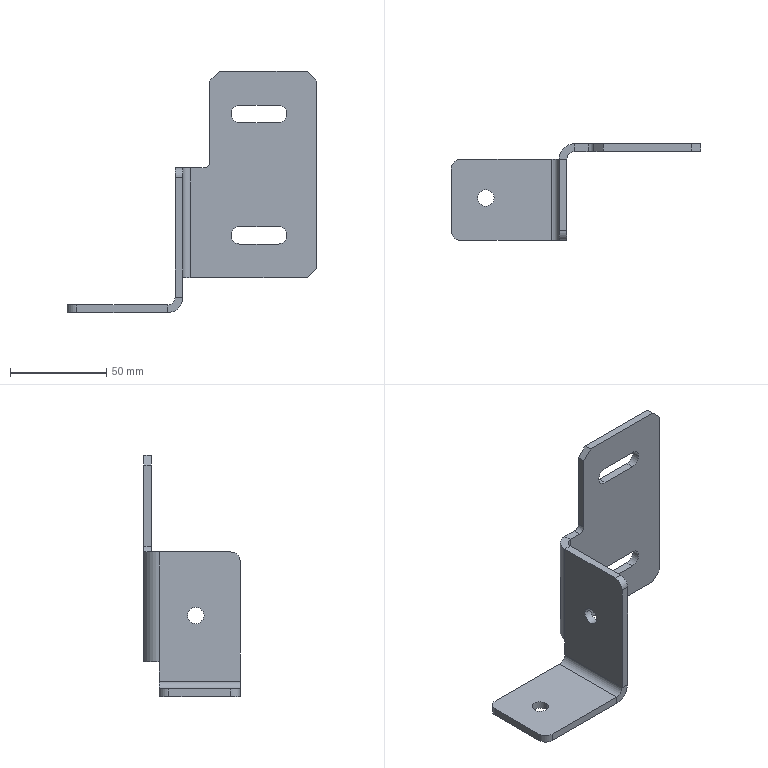Part | SolidWorks | features ICE 4, Fillet 2, Chamfer 1, EdgeFlange 1, FlatPattern 1, SMBaseFlange 1, SheetMetal 1 | 1 solid | 44 faces | box 129.5 x 50 x 125 mm | volume 47149 mm3 | plane 28 | cylinder 16 | commonest cylinder face diameters 8.5 x4 9 x4 10 x3 8 x2 16 x2 6 x1
STEP:
#1=CARTESIAN_POINT('',(-96.75,-28.,-18.));
#2=VERTEX_POINT('',#1);
#3=CARTESIAN_POINT('',(-105.25,-28.,-18.));
#4=VERTEX_POINT('',#3);
#5=CARTESIAN_POINT('',(-101.,-28.,-18.));
#6=DIRECTION('',(0.,0.,-1.));
#7=DIRECTION('',(1.,0.,0.));
#8=AXIS2_PLACEMENT_3D('',#5,#6,#7);
#9=CIRCLE('',#8,4.25);
#10=EDGE_CURVE('',#2,#4,#9,.T.);
#11=ORIENTED_EDGE('',*,*,#10,.T.);
#12=CARTESIAN_POINT('',(-105.25,-28.,-14.));
#13=VERTEX_POINT('',#12);
#14=CARTESIAN_POINT('',(-105.25,-28.,-18.001));
#15=DIRECTION('',(0.,0.,1.));
#16=VECTOR('',#15,1000.);
#17=LINE('',#14,#16);
#18=EDGE_CURVE('',#4,#13,#17,.T.);
#19=ORIENTED_EDGE('',*,*,#18,.T.);
#20=CARTESIAN_POINT('',(-96.75,-28.,-14.));
#21=VERTEX_POINT('',#20);
#22=CARTESIAN_POINT('',(-101.,-28.,-14.));
#23=DIRECTION('',(0.,0.,1.));
#24=DIRECTION('',(1.,0.,0.));
#25=AXIS2_PLACEMENT_3D('',#22,#23,#24);
#26=CIRCLE('',#25,4.25);
#27=EDGE_CURVE('',#13,#21,#26,.T.);
#28=ORIENTED_EDGE('',*,*,#27,.T.);
#29=CARTESIAN_POINT('',(-96.75,-28.,-18.001));
#30=DIRECTION('',(0.,0.,1.));
#31=VECTOR('',#30,1000.);
#32=LINE('',#29,#31);
#33=EDGE_CURVE('',#2,#21,#32,.T.);
#34=ORIENTED_EDGE('',*,*,#33,.F.);
#35=EDGE_LOOP('',(#11,#19,#28,#34));
#36=FACE_OUTER_BOUND('',#35,.T.);
#37=CARTESIAN_POINT('',(-101.,-28.,-18.001));
#38=DIRECTION('',(0.,0.,1.));
#39=DIRECTION('',(1.,0.,0.));
#40=AXIS2_PLACEMENT_3D('',#37,#38,#39);
#41=CYLINDRICAL_SURFACE('',#40,4.25);
#42=ADVANCED_FACE('',(#36),#41,.F.);
#43=CARTESIAN_POINT('',(-59.,-22.75,24.));
#44=VERTEX_POINT('',#43);
#45=CARTESIAN_POINT('',(-59.,-31.25,24.));
#46=VERTEX_POINT('',#45);
#47=CARTESIAN_POINT('',(-59.,-27.,24.));
#48=DIRECTION('',(-1.,0.,0.));
#49=DIRECTION('',(0.,0.,-1.));
#50=AXIS2_PLACEMENT_3D('',#47,#48,#49);
#51=CIRCLE('',#50,4.25);
#52=EDGE_CURVE('',#44,#46,#51,.T.);
#53=ORIENTED_EDGE('',*,*,#52,.F.);
#54=CARTESIAN_POINT('',(-63.,-22.75,24.));
#55=VERTEX_POINT('',#54);
#56=CARTESIAN_POINT('',(10.501,-22.75,24.));
#57=DIRECTION('',(-1.,0.,0.));
#58=VECTOR('',#57,1000.);
#59=LINE('',#56,#58);
#60=EDGE_CURVE('',#44,#55,#59,.T.);
#61=ORIENTED_EDGE('',*,*,#60,.T.);
#62=CARTESIAN_POINT('',(-63.,-31.25,24.));
#63=VERTEX_POINT('',#62);
#64=CARTESIAN_POINT('',(-63.,-27.,24.));
#65=DIRECTION('',(-1.,0.,0.));
#66=DIRECTION('',(0.,-1.,0.));
#67=AXIS2_PLACEMENT_3D('',#64,#65,#66);
#68=CIRCLE('',#67,4.25);
#69=EDGE_CURVE('',#55,#63,#68,.T.);
#70=ORIENTED_EDGE('',*,*,#69,.T.);
#71=CARTESIAN_POINT('',(10.501,-31.25,24.));
#72=DIRECTION('',(-1.,0.,0.));
#73=VECTOR('',#72,1000.);
#74=LINE('',#71,#73);
#75=EDGE_CURVE('',#46,#63,#74,.T.);
#76=ORIENTED_EDGE('',*,*,#75,.F.);
#77=EDGE_LOOP('',(#53,#61,#70,#76));
#78=FACE_OUTER_BOUND('',#77,.T.);
#79=CARTESIAN_POINT('',(10.501,-27.,24.));
#80=DIRECTION('',(-1.,0.,0.));
#81=DIRECTION('',(0.,-1.,0.));
#82=AXIS2_PLACEMENT_3D('',#79,#80,#81);
#83=CYLINDRICAL_SURFACE('',#82,4.25);
#84=ADVANCED_FACE('',(#78),#83,.F.);
#85=CARTESIAN_POINT('',(-48.,-4.,57.));
#86=VERTEX_POINT('',#85);
#87=CARTESIAN_POINT('',(-55.,-4.,57.));
#88=VERTEX_POINT('',#87);
#89=CARTESIAN_POINT('',(-63.,-4.,57.));
#90=DIRECTION('',(-1.,0.,0.));
#91=VECTOR('',#90,1000.);
#92=LINE('',#89,#91);
#93=EDGE_CURVE('',#86,#88,#92,.T.);
#94=ORIENTED_EDGE('',*,*,#93,.F.);
#95=CARTESIAN_POINT('',(-48.,0.,57.));
#96=VERTEX_POINT('',#95);
#97=CARTESIAN_POINT('',(-48.,0.,57.));
#98=DIRECTION('',(0.,1.,0.));
#99=VECTOR('',#98,1000.);
#100=LINE('',#97,#99);
#101=EDGE_CURVE('',#86,#96,#100,.T.);
#102=ORIENTED_EDGE('',*,*,#101,.T.);
#103=CARTESIAN_POINT('',(-55.,0.,57.));
#104=VERTEX_POINT('',#103);
#105=CARTESIAN_POINT('',(-63.,0.,57.));
#106=DIRECTION('',(1.,0.,0.));
#107=VECTOR('',#106,1000.);
#108=LINE('',#105,#107);
#109=EDGE_CURVE('',#104,#96,#108,.T.);
#110=ORIENTED_EDGE('',*,*,#109,.F.);
#111=CARTESIAN_POINT('',(-55.,0.,57.));
#112=DIRECTION('',(0.,-1.,0.));
#113=VECTOR('',#112,1000.);
#114=LINE('',#111,#113);
#115=EDGE_CURVE('',#104,#88,#114,.T.);
#116=ORIENTED_EDGE('',*,*,#115,.T.);
#117=EDGE_LOOP('',(#94,#102,#110,#116));
#118=FACE_OUTER_BOUND('',#117,.T.);
#119=CARTESIAN_POINT('',(-63.,-50.,57.));
#120=DIRECTION('',(0.,0.,1.));
#121=DIRECTION('',(1.,0.,0.));
#122=AXIS2_PLACEMENT_3D('',#119,#120,#121);
#123=PLANE('',#122);
#124=ADVANCED_FACE('',(#118),#123,.T.);
#125=CARTESIAN_POINT('',(-63.,-45.,57.));
#126=VERTEX_POINT('',#125);
#127=CARTESIAN_POINT('',(-63.,-8.,57.));
#128=VERTEX_POINT('',#127);
#129=CARTESIAN_POINT('',(-63.,-50.,57.));
#130=DIRECTION('',(0.,1.,0.));
#131=VECTOR('',#130,1000.);
#132=LINE('',#129,#131);
#133=EDGE_CURVE('',#126,#128,#132,.T.);
#134=ORIENTED_EDGE('',*,*,#133,.F.);
#135=CARTESIAN_POINT('',(-59.,-45.,57.));
#136=VERTEX_POINT('',#135);
#137=CARTESIAN_POINT('',(-63.,-45.,57.));
#138=DIRECTION('',(1.,0.,0.));
#139=VECTOR('',#138,1000.);
#140=LINE('',#137,#139);
#141=EDGE_CURVE('',#126,#136,#140,.T.);
#142=ORIENTED_EDGE('',*,*,#141,.T.);
#143=CARTESIAN_POINT('',(-59.,-8.,57.));
#144=VERTEX_POINT('',#143);
#145=CARTESIAN_POINT('',(-59.,0.,57.));
#146=DIRECTION('',(0.,-1.,0.));
#147=VECTOR('',#146,1000.);
#148=LINE('',#145,#147);
#149=EDGE_CURVE('',#144,#136,#148,.T.);
#150=ORIENTED_EDGE('',*,*,#149,.F.);
#151=CARTESIAN_POINT('',(-59.,-8.,57.));
#152=DIRECTION('',(-1.,0.,0.));
#153=VECTOR('',#152,1000.);
#154=LINE('',#151,#153);
#155=EDGE_CURVE('',#144,#128,#154,.T.);
#156=ORIENTED_EDGE('',*,*,#155,.T.);
#157=EDGE_LOOP('',(#134,#142,#150,#156));
#158=FACE_OUTER_BOUND('',#157,.T.);
#159=CARTESIAN_POINT('',(-63.,-50.,57.));
#160=DIRECTION('',(0.,0.,1.));
#161=DIRECTION('',(1.,0.,0.));
#162=AXIS2_PLACEMENT_3D('',#159,#160,#161);
#163=PLANE('',#162);
#164=ADVANCED_FACE('',(#158),#163,.T.);
#165=CARTESIAN_POINT('',(5.5,-4.,107.));
#166=VERTEX_POINT('',#165);
#167=CARTESIAN_POINT('',(-40.,-4.,107.));
#168=VERTEX_POINT('',#167);
#169=CARTESIAN_POINT('',(-63.,-4.,107.));
#170=DIRECTION('',(-1.,0.,0.));
#171=VECTOR('',#170,1000.);
#172=LINE('',#169,#171);
#173=EDGE_CURVE('',#166,#168,#172,.T.);
#174=ORIENTED_EDGE('',*,*,#173,.F.);
#175=CARTESIAN_POINT('',(5.5,0.,107.));
#176=VERTEX_POINT('',#175);
#177=CARTESIAN_POINT('',(5.5,-8.,107.));
#178=DIRECTION('',(0.,1.,0.));
#179=VECTOR('',#178,1000.);
#180=LINE('',#177,#179);
#181=EDGE_CURVE('',#166,#176,#180,.T.);
#182=ORIENTED_EDGE('',*,*,#181,.T.);
#183=CARTESIAN_POINT('',(-40.,0.,107.));
#184=VERTEX_POINT('',#183);
#185=CARTESIAN_POINT('',(-63.,0.,107.));
#186=DIRECTION('',(-1.,0.,0.));
#187=VECTOR('',#186,1000.);
#188=LINE('',#185,#187);
#189=EDGE_CURVE('',#176,#184,#188,.T.);
#190=ORIENTED_EDGE('',*,*,#189,.T.);
#191=CARTESIAN_POINT('',(-40.,-8.,107.));
#192=DIRECTION('',(0.,-1.,0.));
#193=VECTOR('',#192,1000.);
#194=LINE('',#191,#193);
#195=EDGE_CURVE('',#184,#168,#194,.T.);
#196=ORIENTED_EDGE('',*,*,#195,.T.);
#197=EDGE_LOOP('',(#174,#182,#190,#196));
#198=FACE_OUTER_BOUND('',#197,.T.);
#199=CARTESIAN_POINT('',(-59.,-8.,107.));
#200=DIRECTION('',(0.,0.,1.));
#201=DIRECTION('',(1.,0.,0.));
#202=AXIS2_PLACEMENT_3D('',#199,#200,#201);
#203=PLANE('',#202);
#204=ADVANCED_FACE('',(#198),#203,.T.);
#205=CARTESIAN_POINT('',(-63.,-27.,24.));
#206=DIRECTION('',(-1.,0.,0.));
#207=DIRECTION('',(0.,-1.,0.));
#208=AXIS2_PLACEMENT_3D('',#205,#206,#207);
#209=CIRCLE('',#208,4.25);
#210=EDGE_CURVE('',#63,#55,#209,.T.);
#211=ORIENTED_EDGE('',*,*,#210,.F.);
#212=ORIENTED_EDGE('',*,*,#69,.F.);
#213=EDGE_LOOP('',(#211,#212));
#214=FACE_BOUND('',#213,.T.);
#215=CARTESIAN_POINT('',(-63.,-50.,52.));
#216=VERTEX_POINT('',#215);
#217=CARTESIAN_POINT('',(-63.,-50.,-10.));
#218=VERTEX_POINT('',#217);
#219=CARTESIAN_POINT('',(-63.,-50.,107.));
#220=DIRECTION('',(0.,0.,-1.));
#221=VECTOR('',#220,1000.);
#222=LINE('',#219,#221);
#223=EDGE_CURVE('',#216,#218,#222,.T.);
#224=ORIENTED_EDGE('',*,*,#223,.F.);
#225=CARTESIAN_POINT('',(-63.,-45.,52.));
#226=DIRECTION('',(-1.,0.,0.));
#227=DIRECTION('',(0.,0.,-1.));
#228=AXIS2_PLACEMENT_3D('',#225,#226,#227);
#229=CIRCLE('',#228,5.);
#230=EDGE_CURVE('',#216,#126,#229,.T.);
#231=ORIENTED_EDGE('',*,*,#230,.T.);
#232=ORIENTED_EDGE('',*,*,#133,.T.);
#233=CARTESIAN_POINT('',(-63.,-8.,0.));
#234=VERTEX_POINT('',#233);
#235=CARTESIAN_POINT('',(-63.,-8.,107.));
#236=DIRECTION('',(0.,0.,-1.));
#237=VECTOR('',#236,1000.);
#238=LINE('',#235,#237);
#239=EDGE_CURVE('',#128,#234,#238,.T.);
#240=ORIENTED_EDGE('',*,*,#239,.T.);
#241=CARTESIAN_POINT('',(-63.,-8.,-10.));
#242=VERTEX_POINT('',#241);
#243=CARTESIAN_POINT('',(-63.,-8.,-10.));
#244=DIRECTION('',(0.,0.,1.));
#245=VECTOR('',#244,1000.);
#246=LINE('',#243,#245);
#247=EDGE_CURVE('',#242,#234,#246,.T.);
#248=ORIENTED_EDGE('',*,*,#247,.F.);
#249=CARTESIAN_POINT('',(-63.,-50.,-10.));
#250=DIRECTION('',(0.,1.,0.));
#251=VECTOR('',#250,1000.);
#252=LINE('',#249,#251);
#253=EDGE_CURVE('',#218,#242,#252,.T.);
#254=ORIENTED_EDGE('',*,*,#253,.F.);
#255=EDGE_LOOP('',(#224,#231,#232,#240,#248,#254));
#256=FACE_OUTER_BOUND('',#255,.T.);
#257=CARTESIAN_POINT('',(-63.,0.,107.));
#258=DIRECTION('',(1.,0.,0.));
#259=DIRECTION('',(0.,0.,-1.));
#260=AXIS2_PLACEMENT_3D('',#257,#258,#259);
#261=PLANE('',#260);
#262=ADVANCED_FACE('',(#214,#256),#261,.F.);
#263=CARTESIAN_POINT('',(-59.,-50.,52.));
#264=VERTEX_POINT('',#263);
#265=CARTESIAN_POINT('',(-59.,-50.,-10.));
#266=VERTEX_POINT('',#265);
#267=CARTESIAN_POINT('',(-59.,-50.,107.));
#268=DIRECTION('',(0.,0.,-1.));
#269=VECTOR('',#268,1000.);
#270=LINE('',#267,#269);
#271=EDGE_CURVE('',#264,#266,#270,.T.);
#272=ORIENTED_EDGE('',*,*,#271,.F.);
#273=CARTESIAN_POINT('',(-59.,-50.,52.));
#274=DIRECTION('',(-1.,0.,0.));
#275=VECTOR('',#274,1000.);
#276=LINE('',#273,#275);
#277=EDGE_CURVE('',#264,#216,#276,.T.);
#278=ORIENTED_EDGE('',*,*,#277,.T.);
#279=ORIENTED_EDGE('',*,*,#223,.T.);
#280=CARTESIAN_POINT('',(-63.,-50.,-10.));
#281=DIRECTION('',(1.,0.,0.));
#282=VECTOR('',#281,1000.);
#283=LINE('',#280,#282);
#284=EDGE_CURVE('',#218,#266,#283,.T.);
#285=ORIENTED_EDGE('',*,*,#284,.T.);
#286=EDGE_LOOP('',(#272,#278,#279,#285));
#287=FACE_OUTER_BOUND('',#286,.T.);
#288=CARTESIAN_POINT('',(-59.,-50.,107.));
#289=DIRECTION('',(0.,-1.,0.));
#290=DIRECTION('',(0.,0.,-1.));
#291=AXIS2_PLACEMENT_3D('',#288,#289,#290);
#292=PLANE('',#291);
#293=ADVANCED_FACE('',(#287),#292,.T.);
#294=CARTESIAN_POINT('',(-59.,-27.,24.));
#295=DIRECTION('',(-1.,0.,0.));
#296=DIRECTION('',(0.,0.,-1.));
#297=AXIS2_PLACEMENT_3D('',#294,#295,#296);
#298=CIRCLE('',#297,4.25);
#299=EDGE_CURVE('',#46,#44,#298,.T.);
#300=ORIENTED_EDGE('',*,*,#299,.T.);
#301=ORIENTED_EDGE('',*,*,#52,.T.);
#302=EDGE_LOOP('',(#300,#301));
#303=FACE_BOUND('',#302,.T.);
#304=ORIENTED_EDGE('',*,*,#149,.T.);
#305=CARTESIAN_POINT('',(-59.,-45.,52.));
#306=DIRECTION('',(1.,0.,0.));
#307=DIRECTION('',(0.,0.,-1.));
#308=AXIS2_PLACEMENT_3D('',#305,#306,#307);
#309=CIRCLE('',#308,5.);
#310=EDGE_CURVE('',#136,#264,#309,.T.);
#311=ORIENTED_EDGE('',*,*,#310,.T.);
#312=ORIENTED_EDGE('',*,*,#271,.T.);
#313=CARTESIAN_POINT('',(-59.,-8.,-10.));
#314=VERTEX_POINT('',#313);
#315=CARTESIAN_POINT('',(-59.,-50.,-10.));
#316=DIRECTION('',(0.,1.,0.));
#317=VECTOR('',#316,1000.);
#318=LINE('',#315,#317);
#319=EDGE_CURVE('',#266,#314,#318,.T.);
#320=ORIENTED_EDGE('',*,*,#319,.T.);
#321=CARTESIAN_POINT('',(-59.,-8.,0.));
#322=VERTEX_POINT('',#321);
#323=CARTESIAN_POINT('',(-59.,-8.,-10.));
#324=DIRECTION('',(0.,0.,1.));
#325=VECTOR('',#324,1000.);
#326=LINE('',#323,#325);
#327=EDGE_CURVE('',#314,#322,#326,.T.);
#328=ORIENTED_EDGE('',*,*,#327,.T.);
#329=CARTESIAN_POINT('',(-59.,-8.,107.));
#330=DIRECTION('',(0.,0.,-1.));
#331=VECTOR('',#330,1000.);
#332=LINE('',#329,#331);
#333=EDGE_CURVE('',#144,#322,#332,.T.);
#334=ORIENTED_EDGE('',*,*,#333,.F.);
#335=EDGE_LOOP('',(#304,#311,#312,#320,#328,#334));
#336=FACE_OUTER_BOUND('',#335,.T.);
#337=CARTESIAN_POINT('',(-59.,0.,107.));
#338=DIRECTION('',(1.,0.,0.));
#339=DIRECTION('',(0.,0.,-1.));
#340=AXIS2_PLACEMENT_3D('',#337,#338,#339);
#341=PLANE('',#340);
#342=ADVANCED_FACE('',(#303,#336),#341,.T.);
#343=CARTESIAN_POINT('',(-55.,-4.,0.));
#344=VERTEX_POINT('',#343);
#345=CARTESIAN_POINT('',(-55.,-4.,107.));
#346=DIRECTION('',(0.,0.,-1.));
#347=VECTOR('',#346,1000.);
#348=LINE('',#345,#347);
#349=EDGE_CURVE('',#88,#344,#348,.T.);
#350=ORIENTED_EDGE('',*,*,#349,.F.);
#351=CARTESIAN_POINT('',(-55.,-8.,57.));
#352=DIRECTION('',(0.,0.,1.));
#353=DIRECTION('',(1.,0.,0.));
#354=AXIS2_PLACEMENT_3D('',#351,#352,#353);
#355=CIRCLE('',#354,4.);
#356=EDGE_CURVE('',#88,#144,#355,.T.);
#357=ORIENTED_EDGE('',*,*,#356,.T.);
#358=ORIENTED_EDGE('',*,*,#333,.T.);
#359=CARTESIAN_POINT('',(-55.,-8.,0.));
#360=DIRECTION('',(0.,0.,1.));
#361=DIRECTION('',(1.,0.,0.));
#362=AXIS2_PLACEMENT_3D('',#359,#360,#361);
#363=CIRCLE('',#362,4.);
#364=EDGE_CURVE('',#344,#322,#363,.T.);
#365=ORIENTED_EDGE('',*,*,#364,.F.);
#366=EDGE_LOOP('',(#350,#357,#358,#365));
#367=FACE_OUTER_BOUND('',#366,.T.);
#368=CARTESIAN_POINT('',(-55.,-8.,107.));
#369=DIRECTION('',(0.,0.,-1.));
#370=DIRECTION('',(-1.,0.,0.));
#371=AXIS2_PLACEMENT_3D('',#368,#369,#370);
#372=CYLINDRICAL_SURFACE('',#371,4.);
#373=ADVANCED_FACE('',(#367),#372,.F.);
#374=CARTESIAN_POINT('',(-29.5,-4.,89.5));
#375=VERTEX_POINT('',#374);
#376=CARTESIAN_POINT('',(-29.5,-4.,80.5));
#377=VERTEX_POINT('',#376);
#378=CARTESIAN_POINT('',(-29.5,-4.,85.));
#379=DIRECTION('',(0.,-1.,0.));
#380=DIRECTION('',(0.,0.,-1.));
#381=AXIS2_PLACEMENT_3D('',#378,#379,#380);
#382=CIRCLE('',#381,4.5);
#383=EDGE_CURVE('',#375,#377,#382,.T.);
#384=ORIENTED_EDGE('',*,*,#383,.F.);
#385=CARTESIAN_POINT('',(-9.5,-4.,89.5));
#386=VERTEX_POINT('',#385);
#387=CARTESIAN_POINT('',(-29.5,-4.,89.5));
#388=DIRECTION('',(-1.,0.,0.));
#389=VECTOR('',#388,1000.);
#390=LINE('',#387,#389);
#391=EDGE_CURVE('',#386,#375,#390,.T.);
#392=ORIENTED_EDGE('',*,*,#391,.F.);
#393=CARTESIAN_POINT('',(-9.5,-4.,80.5));
#394=VERTEX_POINT('',#393);
#395=CARTESIAN_POINT('',(-9.5,-4.,85.));
#396=DIRECTION('',(0.,-1.,0.));
#397=DIRECTION('',(0.,0.,-1.));
#398=AXIS2_PLACEMENT_3D('',#395,#396,#397);
#399=CIRCLE('',#398,4.5);
#400=EDGE_CURVE('',#394,#386,#399,.T.);
#401=ORIENTED_EDGE('',*,*,#400,.F.);
#402=CARTESIAN_POINT('',(-29.5,-4.,80.5));
#403=DIRECTION('',(1.,0.,0.));
#404=VECTOR('',#403,1000.);
#405=LINE('',#402,#404);
#406=EDGE_CURVE('',#377,#394,#405,.T.);
#407=ORIENTED_EDGE('',*,*,#406,.F.);
#408=EDGE_LOOP('',(#384,#392,#401,#407));
#409=FACE_BOUND('',#408,.T.);
#410=CARTESIAN_POINT('',(-29.5,-4.,26.5));
#411=VERTEX_POINT('',#410);
#412=CARTESIAN_POINT('',(-29.5,-4.,17.5));
#413=VERTEX_POINT('',#412);
#414=CARTESIAN_POINT('',(-29.5,-4.,22.));
#415=DIRECTION('',(0.,-1.,0.));
#416=DIRECTION('',(0.,0.,-1.));
#417=AXIS2_PLACEMENT_3D('',#414,#415,#416);
#418=CIRCLE('',#417,4.5);
#419=EDGE_CURVE('',#411,#413,#418,.T.);
#420=ORIENTED_EDGE('',*,*,#419,.F.);
#421=CARTESIAN_POINT('',(-9.5,-4.,26.5));
#422=VERTEX_POINT('',#421);
#423=CARTESIAN_POINT('',(-29.5,-4.,26.5));
#424=DIRECTION('',(-1.,0.,0.));
#425=VECTOR('',#424,1000.);
#426=LINE('',#423,#425);
#427=EDGE_CURVE('',#422,#411,#426,.T.);
#428=ORIENTED_EDGE('',*,*,#427,.F.);
#429=CARTESIAN_POINT('',(-9.5,-4.,17.5));
#430=VERTEX_POINT('',#429);
#431=CARTESIAN_POINT('',(-9.5,-4.,22.));
#432=DIRECTION('',(0.,-1.,0.));
#433=DIRECTION('',(0.,0.,-1.));
#434=AXIS2_PLACEMENT_3D('',#431,#432,#433);
#435=CIRCLE('',#434,4.5);
#436=EDGE_CURVE('',#430,#422,#435,.T.);
#437=ORIENTED_EDGE('',*,*,#436,.F.);
#438=CARTESIAN_POINT('',(-29.5,-4.,17.5));
#439=DIRECTION('',(1.,0.,0.));
#440=VECTOR('',#439,1000.);
#441=LINE('',#438,#440);
#442=EDGE_CURVE('',#413,#430,#441,.T.);
#443=ORIENTED_EDGE('',*,*,#442,.F.);
#444=EDGE_LOOP('',(#420,#428,#437,#443));
#445=FACE_BOUND('',#444,.T.);
#446=CARTESIAN_POINT('',(5.5,-4.,0.));
#447=VERTEX_POINT('',#446);
#448=CARTESIAN_POINT('',(-63.,-4.,0.));
#449=DIRECTION('',(-1.,0.,0.));
#450=VECTOR('',#449,1000.);
#451=LINE('',#448,#450);
#452=EDGE_CURVE('',#447,#344,#451,.T.);
#453=ORIENTED_EDGE('',*,*,#452,.F.);
#454=CARTESIAN_POINT('',(10.5,-4.,5.));
#455=VERTEX_POINT('',#454);
#456=CARTESIAN_POINT('',(24.75,-4.,19.25));
#457=DIRECTION('',(0.7071,0.,0.7071));
#458=VECTOR('',#457,1000.);
#459=LINE('',#456,#458);
#460=EDGE_CURVE('',#447,#455,#459,.T.);
#461=ORIENTED_EDGE('',*,*,#460,.T.);
#462=CARTESIAN_POINT('',(10.5,-4.,102.));
#463=VERTEX_POINT('',#462);
#464=CARTESIAN_POINT('',(10.5,-4.,107.));
#465=DIRECTION('',(0.,0.,-1.));
#466=VECTOR('',#465,1000.);
#467=LINE('',#464,#466);
#468=EDGE_CURVE('',#463,#455,#467,.T.);
#469=ORIENTED_EDGE('',*,*,#468,.F.);
#470=CARTESIAN_POINT('',(-28.75,-4.,141.25));
#471=DIRECTION('',(-0.7071,0.,0.7071));
#472=VECTOR('',#471,1000.);
#473=LINE('',#470,#472);
#474=EDGE_CURVE('',#463,#166,#473,.T.);
#475=ORIENTED_EDGE('',*,*,#474,.T.);
#476=ORIENTED_EDGE('',*,*,#173,.T.);
#477=CARTESIAN_POINT('',(-45.,-4.,102.));
#478=VERTEX_POINT('',#477);
#479=CARTESIAN_POINT('',(-51.5,-4.,95.5));
#480=DIRECTION('',(-0.7071,0.,-0.7071));
#481=VECTOR('',#480,1000.);
#482=LINE('',#479,#481);
#483=EDGE_CURVE('',#168,#478,#482,.T.);
#484=ORIENTED_EDGE('',*,*,#483,.T.);
#485=CARTESIAN_POINT('',(-45.,-4.,60.));
#486=VERTEX_POINT('',#485);
#487=CARTESIAN_POINT('',(-45.,-4.,107.));
#488=DIRECTION('',(0.,0.,-1.));
#489=VECTOR('',#488,1000.);
#490=LINE('',#487,#489);
#491=EDGE_CURVE('',#478,#486,#490,.T.);
#492=ORIENTED_EDGE('',*,*,#491,.T.);
#493=CARTESIAN_POINT('',(-48.,-4.,60.));
#494=DIRECTION('',(0.,1.,0.));
#495=DIRECTION('',(0.,0.,-1.));
#496=AXIS2_PLACEMENT_3D('',#493,#494,#495);
#497=CIRCLE('',#496,3.);
#498=EDGE_CURVE('',#486,#86,#497,.T.);
#499=ORIENTED_EDGE('',*,*,#498,.T.);
#500=ORIENTED_EDGE('',*,*,#93,.T.);
#501=ORIENTED_EDGE('',*,*,#349,.T.);
#502=EDGE_LOOP('',(#453,#461,#469,#475,#476,#484,#492,#499,#500,#501));
#503=FACE_OUTER_BOUND('',#502,.T.);
#504=CARTESIAN_POINT('',(-63.,-4.,107.));
#505=DIRECTION('',(0.,-1.,0.));
#506=DIRECTION('',(0.,0.,-1.));
#507=AXIS2_PLACEMENT_3D('',#504,#505,#506);
#508=PLANE('',#507);
#509=ADVANCED_FACE('',(#409,#445,#503),#508,.T.);
#510=CARTESIAN_POINT('',(-29.5,0.,89.5));
#511=VERTEX_POINT('',#510);
#512=CARTESIAN_POINT('',(-9.5,0.,89.5));
#513=VERTEX_POINT('',#512);
#514=CARTESIAN_POINT('',(-29.5,0.,89.5));
#515=DIRECTION('',(1.,0.,0.));
#516=VECTOR('',#515,1000.);
#517=LINE('',#514,#516);
#518=EDGE_CURVE('',#511,#513,#517,.T.);
#519=ORIENTED_EDGE('',*,*,#518,.F.);
#520=CARTESIAN_POINT('',(-29.5,0.,80.5));
#521=VERTEX_POINT('',#520);
#522=CARTESIAN_POINT('',(-29.5,0.,85.));
#523=DIRECTION('',(0.,1.,0.));
#524=DIRECTION('',(0.,0.,-1.));
#525=AXIS2_PLACEMENT_3D('',#522,#523,#524);
#526=CIRCLE('',#525,4.5);
#527=EDGE_CURVE('',#521,#511,#526,.T.);
#528=ORIENTED_EDGE('',*,*,#527,.F.);
#529=CARTESIAN_POINT('',(-9.5,0.,80.5));
#530=VERTEX_POINT('',#529);
#531=CARTESIAN_POINT('',(-29.5,0.,80.5));
#532=DIRECTION('',(-1.,0.,0.));
#533=VECTOR('',#532,1000.);
#534=LINE('',#531,#533);
#535=EDGE_CURVE('',#530,#521,#534,.T.);
#536=ORIENTED_EDGE('',*,*,#535,.F.);
#537=CARTESIAN_POINT('',(-9.5,0.,85.));
#538=DIRECTION('',(0.,1.,0.));
#539=DIRECTION('',(0.,0.,-1.));
#540=AXIS2_PLACEMENT_3D('',#537,#538,#539);
#541=CIRCLE('',#540,4.5);
#542=EDGE_CURVE('',#513,#530,#541,.T.);
#543=ORIENTED_EDGE('',*,*,#542,.F.);
#544=EDGE_LOOP('',(#519,#528,#536,#543));
#545=FACE_BOUND('',#544,.T.);
#546=CARTESIAN_POINT('',(-29.5,0.,26.5));
#547=VERTEX_POINT('',#546);
#548=CARTESIAN_POINT('',(-9.5,0.,26.5));
#549=VERTEX_POINT('',#548);
#550=CARTESIAN_POINT('',(-29.5,0.,26.5));
#551=DIRECTION('',(1.,0.,0.));
#552=VECTOR('',#551,1000.);
#553=LINE('',#550,#552);
#554=EDGE_CURVE('',#547,#549,#553,.T.);
#555=ORIENTED_EDGE('',*,*,#554,.F.);
#556=CARTESIAN_POINT('',(-29.5,0.,17.5));
#557=VERTEX_POINT('',#556);
#558=CARTESIAN_POINT('',(-29.5,0.,22.));
#559=DIRECTION('',(0.,1.,0.));
#560=DIRECTION('',(0.,0.,-1.));
#561=AXIS2_PLACEMENT_3D('',#558,#559,#560);
#562=CIRCLE('',#561,4.5);
#563=EDGE_CURVE('',#557,#547,#562,.T.);
#564=ORIENTED_EDGE('',*,*,#563,.F.);
#565=CARTESIAN_POINT('',(-9.5,0.,17.5));
#566=VERTEX_POINT('',#565);
#567=CARTESIAN_POINT('',(-29.5,0.,17.5));
#568=DIRECTION('',(-1.,0.,0.));
#569=VECTOR('',#568,1000.);
#570=LINE('',#567,#569);
#571=EDGE_CURVE('',#566,#557,#570,.T.);
#572=ORIENTED_EDGE('',*,*,#571,.F.);
#573=CARTESIAN_POINT('',(-9.5,0.,22.));
#574=DIRECTION('',(0.,1.,0.));
#575=DIRECTION('',(0.,0.,-1.));
#576=AXIS2_PLACEMENT_3D('',#573,#574,#575);
#577=CIRCLE('',#576,4.5);
#578=EDGE_CURVE('',#549,#566,#577,.T.);
#579=ORIENTED_EDGE('',*,*,#578,.F.);
#580=EDGE_LOOP('',(#555,#564,#572,#579));
#581=FACE_BOUND('',#580,.T.);
#582=CARTESIAN_POINT('',(10.5,0.,102.));
#583=VERTEX_POINT('',#582);
#584=CARTESIAN_POINT('',(10.5,0.,5.));
#585=VERTEX_POINT('',#584);
#586=CARTESIAN_POINT('',(10.5,0.,107.));
#587=DIRECTION('',(0.,0.,-1.));
#588=VECTOR('',#587,1000.);
#589=LINE('',#586,#588);
#590=EDGE_CURVE('',#583,#585,#589,.T.);
#591=ORIENTED_EDGE('',*,*,#590,.T.);
#592=CARTESIAN_POINT('',(5.5,0.,0.));
#593=VERTEX_POINT('',#592);
#594=CARTESIAN_POINT('',(5.5,0.,0.));
#595=DIRECTION('',(-0.7071,0.,-0.7071));
#596=VECTOR('',#595,1000.);
#597=LINE('',#594,#596);
#598=EDGE_CURVE('',#585,#593,#597,.T.);
#599=ORIENTED_EDGE('',*,*,#598,.T.);
#600=CARTESIAN_POINT('',(-55.,0.,0.));
#601=VERTEX_POINT('',#600);
#602=CARTESIAN_POINT('',(-63.,0.,0.));
#603=DIRECTION('',(-1.,0.,0.));
#604=VECTOR('',#603,1000.);
#605=LINE('',#602,#604);
#606=EDGE_CURVE('',#593,#601,#605,.T.);
#607=ORIENTED_EDGE('',*,*,#606,.T.);
#608=CARTESIAN_POINT('',(-55.,0.,107.));
#609=DIRECTION('',(0.,0.,-1.));
#610=VECTOR('',#609,1000.);
#611=LINE('',#608,#610);
#612=EDGE_CURVE('',#104,#601,#611,.T.);
#613=ORIENTED_EDGE('',*,*,#612,.F.);
#614=ORIENTED_EDGE('',*,*,#109,.T.);
#615=CARTESIAN_POINT('',(-45.,0.,60.));
#616=VERTEX_POINT('',#615);
#617=CARTESIAN_POINT('',(-48.,0.,60.));
#618=DIRECTION('',(0.,-1.,0.));
#619=DIRECTION('',(0.,0.,-1.));
#620=AXIS2_PLACEMENT_3D('',#617,#618,#619);
#621=CIRCLE('',#620,3.);
#622=EDGE_CURVE('',#96,#616,#621,.T.);
#623=ORIENTED_EDGE('',*,*,#622,.T.);
#624=CARTESIAN_POINT('',(-45.,0.,102.));
#625=VERTEX_POINT('',#624);
#626=CARTESIAN_POINT('',(-45.,0.,107.));
#627=DIRECTION('',(0.,0.,1.));
#628=VECTOR('',#627,1000.);
#629=LINE('',#626,#628);
#630=EDGE_CURVE('',#616,#625,#629,.T.);
#631=ORIENTED_EDGE('',*,*,#630,.T.);
#632=CARTESIAN_POINT('',(-45.,0.,102.));
#633=DIRECTION('',(0.7071,0.,0.7071));
#634=VECTOR('',#633,1000.);
#635=LINE('',#632,#634);
#636=EDGE_CURVE('',#625,#184,#635,.T.);
#637=ORIENTED_EDGE('',*,*,#636,.T.);
#638=ORIENTED_EDGE('',*,*,#189,.F.);
#639=CARTESIAN_POINT('',(10.5,0.,102.));
#640=DIRECTION('',(0.7071,0.,-0.7071));
#641=VECTOR('',#640,1000.);
#642=LINE('',#639,#641);
#643=EDGE_CURVE('',#176,#583,#642,.T.);
#644=ORIENTED_EDGE('',*,*,#643,.T.);
#645=EDGE_LOOP('',(#591,#599,#607,#613,#614,#623,#631,#637,#638,#644));
#646=FACE_OUTER_BOUND('',#645,.T.);
#647=CARTESIAN_POINT('',(-63.,0.,107.));
#648=DIRECTION('',(0.,-1.,0.));
#649=DIRECTION('',(0.,0.,-1.));
#650=AXIS2_PLACEMENT_3D('',#647,#648,#649);
#651=PLANE('',#650);
#652=ADVANCED_FACE('',(#545,#581,#646),#651,.F.);
#653=CARTESIAN_POINT('',(-55.,-8.,57.));
#654=DIRECTION('',(0.,0.,1.));
#655=DIRECTION('',(1.,0.,0.));
#656=AXIS2_PLACEMENT_3D('',#653,#654,#655);
#657=CIRCLE('',#656,8.);
#658=EDGE_CURVE('',#104,#128,#657,.T.);
#659=ORIENTED_EDGE('',*,*,#658,.F.);
#660=ORIENTED_EDGE('',*,*,#612,.T.);
#661=CARTESIAN_POINT('',(-55.,-8.,0.));
#662=DIRECTION('',(0.,0.,1.));
#663=DIRECTION('',(-1.,0.,0.));
#664=AXIS2_PLACEMENT_3D('',#661,#662,#663);
#665=CIRCLE('',#664,8.);
#666=EDGE_CURVE('',#601,#234,#665,.T.);
#667=ORIENTED_EDGE('',*,*,#666,.T.);
#668=ORIENTED_EDGE('',*,*,#239,.F.);
#669=EDGE_LOOP('',(#659,#660,#667,#668));
#670=FACE_OUTER_BOUND('',#669,.T.);
#671=CARTESIAN_POINT('',(-55.,-8.,107.));
#672=DIRECTION('',(0.,0.,-1.));
#673=DIRECTION('',(-1.,0.,0.));
#674=AXIS2_PLACEMENT_3D('',#671,#672,#673);
#675=CYLINDRICAL_SURFACE('',#674,8.);
#676=ADVANCED_FACE('',(#670),#675,.T.);
#677=CARTESIAN_POINT('',(-63.,-8.,0.));
#678=DIRECTION('',(1.,0.,0.));
#679=VECTOR('',#678,1000.);
#680=LINE('',#677,#679);
#681=EDGE_CURVE('',#234,#322,#680,.T.);
#682=ORIENTED_EDGE('',*,*,#681,.F.);
#683=ORIENTED_EDGE('',*,*,#666,.F.);
#684=CARTESIAN_POINT('',(-55.,-4.,0.));
#685=DIRECTION('',(0.,1.,0.));
#686=VECTOR('',#685,1000.);
#687=LINE('',#684,#686);
#688=EDGE_CURVE('',#344,#601,#687,.T.);
#689=ORIENTED_EDGE('',*,*,#688,.F.);
#690=ORIENTED_EDGE('',*,*,#364,.T.);
#691=EDGE_LOOP('',(#682,#683,#689,#690));
#692=FACE_OUTER_BOUND('',#691,.T.);
#693=CARTESIAN_POINT('',(-63.,-8.,0.));
#694=DIRECTION('',(0.,0.,-1.));
#695=DIRECTION('',(-1.,0.,0.));
#696=AXIS2_PLACEMENT_3D('',#693,#694,#695);
#697=PLANE('',#696);
#698=ADVANCED_FACE('',(#692),#697,.T.);
#699=ORIENTED_EDGE('',*,*,#468,.T.);
#700=CARTESIAN_POINT('',(10.5,0.,5.));
#701=DIRECTION('',(0.,1.,0.));
#702=VECTOR('',#701,1000.);
#703=LINE('',#700,#702);
#704=EDGE_CURVE('',#455,#585,#703,.T.);
#705=ORIENTED_EDGE('',*,*,#704,.T.);
#706=ORIENTED_EDGE('',*,*,#590,.F.);
#707=CARTESIAN_POINT('',(10.5,0.,102.));
#708=DIRECTION('',(0.,-1.,0.));
#709=VECTOR('',#708,1000.);
#710=LINE('',#707,#709);
#711=EDGE_CURVE('',#583,#463,#710,.T.);
#712=ORIENTED_EDGE('',*,*,#711,.T.);
#713=EDGE_LOOP('',(#699,#705,#706,#712));
#714=FACE_OUTER_BOUND('',#713,.T.);
#715=CARTESIAN_POINT('',(10.5,0.,107.));
#716=DIRECTION('',(1.,0.,0.));
#717=DIRECTION('',(0.,1.,0.));
#718=AXIS2_PLACEMENT_3D('',#715,#716,#717);
#719=PLANE('',#718);
#720=ADVANCED_FACE('',(#714),#719,.T.);
#721=ORIENTED_EDGE('',*,*,#606,.F.);
#722=CARTESIAN_POINT('',(5.5,-4.,0.));
#723=DIRECTION('',(0.,-1.,0.));
#724=VECTOR('',#723,1000.);
#725=LINE('',#722,#724);
#726=EDGE_CURVE('',#593,#447,#725,.T.);
#727=ORIENTED_EDGE('',*,*,#726,.T.);
#728=ORIENTED_EDGE('',*,*,#452,.T.);
#729=ORIENTED_EDGE('',*,*,#688,.T.);
#730=EDGE_LOOP('',(#721,#727,#728,#729));
#731=FACE_OUTER_BOUND('',#730,.T.);
#732=CARTESIAN_POINT('',(-55.,-8.,0.));
#733=DIRECTION('',(0.,0.,1.));
#734=DIRECTION('',(1.,0.,0.));
#735=AXIS2_PLACEMENT_3D('',#732,#733,#734);
#736=PLANE('',#735);
#737=ADVANCED_FACE('',(#731),#736,.F.);
#738=ORIENTED_EDGE('',*,*,#115,.F.);
#739=ORIENTED_EDGE('',*,*,#658,.T.);
#740=ORIENTED_EDGE('',*,*,#155,.F.);
#741=ORIENTED_EDGE('',*,*,#356,.F.);
#742=EDGE_LOOP('',(#738,#739,#740,#741));
#743=FACE_OUTER_BOUND('',#742,.T.);
#744=CARTESIAN_POINT('',(-63.,-50.,57.));
#745=DIRECTION('',(0.,0.,1.));
#746=DIRECTION('',(1.,0.,0.));
#747=AXIS2_PLACEMENT_3D('',#744,#745,#746);
#748=PLANE('',#747);
#749=ADVANCED_FACE('',(#743),#748,.T.);
#750=ORIENTED_EDGE('',*,*,#630,.F.);
#751=CARTESIAN_POINT('',(-45.,-4.,60.));
#752=DIRECTION('',(0.,-1.,0.));
#753=VECTOR('',#752,1000.);
#754=LINE('',#751,#753);
#755=EDGE_CURVE('',#616,#486,#754,.T.);
#756=ORIENTED_EDGE('',*,*,#755,.T.);
#757=ORIENTED_EDGE('',*,*,#491,.F.);
#758=CARTESIAN_POINT('',(-45.,-50.,102.));
#759=DIRECTION('',(0.,1.,0.));
#760=VECTOR('',#759,1000.);
#761=LINE('',#758,#760);
#762=EDGE_CURVE('',#478,#625,#761,.T.);
#763=ORIENTED_EDGE('',*,*,#762,.T.);
#764=EDGE_LOOP('',(#750,#756,#757,#763));
#765=FACE_OUTER_BOUND('',#764,.T.);
#766=CARTESIAN_POINT('',(-45.,-50.,107.));
#767=DIRECTION('',(-1.,0.,0.));
#768=DIRECTION('',(0.,0.,1.));
#769=AXIS2_PLACEMENT_3D('',#766,#767,#768);
#770=PLANE('',#769);
#771=ADVANCED_FACE('',(#765),#770,.T.);
#772=ORIENTED_EDGE('',*,*,#327,.F.);
#773=CARTESIAN_POINT('',(-63.,-8.,-10.));
#774=DIRECTION('',(1.,0.,0.));
#775=VECTOR('',#774,1000.);
#776=LINE('',#773,#775);
#777=EDGE_CURVE('',#242,#314,#776,.T.);
#778=ORIENTED_EDGE('',*,*,#777,.F.);
#779=ORIENTED_EDGE('',*,*,#247,.T.);
#780=ORIENTED_EDGE('',*,*,#681,.T.);
#781=EDGE_LOOP('',(#772,#778,#779,#780));
#782=FACE_OUTER_BOUND('',#781,.T.);
#783=CARTESIAN_POINT('',(-63.,-8.,-10.));
#784=DIRECTION('',(0.,-1.,0.));
#785=DIRECTION('',(1.,0.,0.));
#786=AXIS2_PLACEMENT_3D('',#783,#784,#785);
#787=PLANE('',#786);
#788=ADVANCED_FACE('',(#782),#787,.F.);
#789=CARTESIAN_POINT('',(-67.,-8.,-14.));
#790=VERTEX_POINT('',#789);
#791=CARTESIAN_POINT('',(-67.,-8.,-18.));
#792=VERTEX_POINT('',#791);
#793=CARTESIAN_POINT('',(-67.,-8.,-18.));
#794=DIRECTION('',(0.,0.,-1.));
#795=VECTOR('',#794,1000.);
#796=LINE('',#793,#795);
#797=EDGE_CURVE('',#790,#792,#796,.T.);
#798=ORIENTED_EDGE('',*,*,#797,.F.);
#799=CARTESIAN_POINT('',(-67.,-8.,-10.));
#800=DIRECTION('',(0.,1.,0.));
#801=DIRECTION('',(0.,0.,-1.));
#802=AXIS2_PLACEMENT_3D('',#799,#800,#801);
#803=CIRCLE('',#802,4.);
#804=EDGE_CURVE('',#242,#790,#803,.T.);
#805=ORIENTED_EDGE('',*,*,#804,.F.);
#806=ORIENTED_EDGE('',*,*,#777,.T.);
#807=CARTESIAN_POINT('',(-67.,-8.,-10.));
#808=DIRECTION('',(0.,1.,0.));
#809=DIRECTION('',(0.,0.,-1.));
#810=AXIS2_PLACEMENT_3D('',#807,#808,#809);
#811=CIRCLE('',#810,8.);
#812=EDGE_CURVE('',#314,#792,#811,.T.);
#813=ORIENTED_EDGE('',*,*,#812,.T.);
#814=EDGE_LOOP('',(#798,#805,#806,#813));
#815=FACE_OUTER_BOUND('',#814,.T.);
#816=CARTESIAN_POINT('',(-67.,-8.,-10.));
#817=DIRECTION('',(0.,1.,0.));
#818=DIRECTION('',(0.,0.,1.));
#819=AXIS2_PLACEMENT_3D('',#816,#817,#818);
#820=PLANE('',#819);
#821=ADVANCED_FACE('',(#815),#820,.T.);
#822=CARTESIAN_POINT('',(-67.,-50.,-14.));
#823=VERTEX_POINT('',#822);
#824=CARTESIAN_POINT('',(-67.,-50.,-10.));
#825=DIRECTION('',(0.,-1.,0.));
#826=DIRECTION('',(0.,0.,-1.));
#827=AXIS2_PLACEMENT_3D('',#824,#825,#826);
#828=CIRCLE('',#827,4.);
#829=EDGE_CURVE('',#823,#218,#828,.T.);
#830=ORIENTED_EDGE('',*,*,#829,.F.);
#831=CARTESIAN_POINT('',(-67.,-50.,-18.));
#832=VERTEX_POINT('',#831);
#833=CARTESIAN_POINT('',(-67.,-50.,-14.));
#834=DIRECTION('',(0.,0.,-1.));
#835=VECTOR('',#834,1000.);
#836=LINE('',#833,#835);
#837=EDGE_CURVE('',#823,#832,#836,.T.);
#838=ORIENTED_EDGE('',*,*,#837,.T.);
#839=CARTESIAN_POINT('',(-67.,-50.,-10.));
#840=DIRECTION('',(0.,-1.,0.));
#841=DIRECTION('',(0.,0.,-1.));
#842=AXIS2_PLACEMENT_3D('',#839,#840,#841);
#843=CIRCLE('',#842,8.);
#844=EDGE_CURVE('',#832,#266,#843,.T.);
#845=ORIENTED_EDGE('',*,*,#844,.T.);
#846=ORIENTED_EDGE('',*,*,#284,.F.);
#847=EDGE_LOOP('',(#830,#838,#845,#846));
#848=FACE_OUTER_BOUND('',#847,.T.);
#849=CARTESIAN_POINT('',(-67.,-50.,-10.));
#850=DIRECTION('',(0.,1.,0.));
#851=DIRECTION('',(0.,0.,1.));
#852=AXIS2_PLACEMENT_3D('',#849,#850,#851);
#853=PLANE('',#852);
#854=ADVANCED_FACE('',(#848),#853,.F.);
#855=ORIENTED_EDGE('',*,*,#319,.F.);
#856=ORIENTED_EDGE('',*,*,#844,.F.);
#857=CARTESIAN_POINT('',(-67.,-8.,-18.));
#858=DIRECTION('',(0.,1.,0.));
#859=VECTOR('',#858,1000.);
#860=LINE('',#857,#859);
#861=EDGE_CURVE('',#832,#792,#860,.T.);
#862=ORIENTED_EDGE('',*,*,#861,.T.);
#863=ORIENTED_EDGE('',*,*,#812,.F.);
#864=EDGE_LOOP('',(#855,#856,#862,#863));
#865=FACE_OUTER_BOUND('',#864,.T.);
#866=CARTESIAN_POINT('',(-67.,-50.,-10.));
#867=DIRECTION('',(0.,-1.,0.));
#868=DIRECTION('',(0.,0.,-1.));
#869=AXIS2_PLACEMENT_3D('',#866,#867,#868);
#870=CYLINDRICAL_SURFACE('',#869,8.);
#871=ADVANCED_FACE('',(#865),#870,.T.);
#872=ORIENTED_EDGE('',*,*,#253,.T.);
#873=ORIENTED_EDGE('',*,*,#804,.T.);
#874=CARTESIAN_POINT('',(-67.,-8.,-14.));
#875=DIRECTION('',(0.,-1.,0.));
#876=VECTOR('',#875,1000.);
#877=LINE('',#874,#876);
#878=EDGE_CURVE('',#790,#823,#877,.T.);
#879=ORIENTED_EDGE('',*,*,#878,.T.);
#880=ORIENTED_EDGE('',*,*,#829,.T.);
#881=EDGE_LOOP('',(#872,#873,#879,#880));
#882=FACE_OUTER_BOUND('',#881,.T.);
#883=CARTESIAN_POINT('',(-67.,-50.,-10.));
#884=DIRECTION('',(0.,-1.,0.));
#885=DIRECTION('',(0.,0.,-1.));
#886=AXIS2_PLACEMENT_3D('',#883,#884,#885);
#887=CYLINDRICAL_SURFACE('',#886,4.);
#888=ADVANCED_FACE('',(#882),#887,.F.);
#889=CARTESIAN_POINT('',(-114.,-8.,-18.));
#890=VERTEX_POINT('',#889);
#891=CARTESIAN_POINT('',(0.,-8.,-18.));
#892=DIRECTION('',(1.,0.,0.));
#893=VECTOR('',#892,1000.);
#894=LINE('',#891,#893);
#895=EDGE_CURVE('',#890,#792,#894,.T.);
#896=ORIENTED_EDGE('',*,*,#895,.F.);
#897=CARTESIAN_POINT('',(-114.,-8.,-14.));
#898=VERTEX_POINT('',#897);
#899=CARTESIAN_POINT('',(-114.,-8.,-18.));
#900=DIRECTION('',(0.,0.,1.));
#901=VECTOR('',#900,1000.);
#902=LINE('',#899,#901);
#903=EDGE_CURVE('',#890,#898,#902,.T.);
#904=ORIENTED_EDGE('',*,*,#903,.T.);
#905=CARTESIAN_POINT('',(-63.,-8.,-14.));
#906=DIRECTION('',(1.,0.,0.));
#907=VECTOR('',#906,1000.);
#908=LINE('',#905,#907);
#909=EDGE_CURVE('',#898,#790,#908,.T.);
#910=ORIENTED_EDGE('',*,*,#909,.T.);
#911=ORIENTED_EDGE('',*,*,#797,.T.);
#912=EDGE_LOOP('',(#896,#904,#910,#911));
#913=FACE_OUTER_BOUND('',#912,.T.);
#914=CARTESIAN_POINT('',(-63.,-8.,-18.));
#915=DIRECTION('',(0.,-1.,0.));
#916=DIRECTION('',(1.,0.,0.));
#917=AXIS2_PLACEMENT_3D('',#914,#915,#916);
#918=PLANE('',#917);
#919=ADVANCED_FACE('',(#913),#918,.F.);
#920=CARTESIAN_POINT('',(-114.,-50.,-14.));
#921=VERTEX_POINT('',#920);
#922=CARTESIAN_POINT('',(-119.,-50.,-14.));
#923=DIRECTION('',(-1.,0.,0.));
#924=VECTOR('',#923,1000.);
#925=LINE('',#922,#924);
#926=EDGE_CURVE('',#823,#921,#925,.T.);
#927=ORIENTED_EDGE('',*,*,#926,.T.);
#928=CARTESIAN_POINT('',(-114.,-50.,-18.));
#929=VERTEX_POINT('',#928);
#930=CARTESIAN_POINT('',(-114.,-50.,-18.));
#931=DIRECTION('',(0.,0.,-1.));
#932=VECTOR('',#931,1000.);
#933=LINE('',#930,#932);
#934=EDGE_CURVE('',#921,#929,#933,.T.);
#935=ORIENTED_EDGE('',*,*,#934,.T.);
#936=CARTESIAN_POINT('',(0.,-50.,-18.));
#937=DIRECTION('',(-1.,0.,0.));
#938=VECTOR('',#937,1000.);
#939=LINE('',#936,#938);
#940=EDGE_CURVE('',#832,#929,#939,.T.);
#941=ORIENTED_EDGE('',*,*,#940,.F.);
#942=ORIENTED_EDGE('',*,*,#837,.F.);
#943=EDGE_LOOP('',(#927,#935,#941,#942));
#944=FACE_OUTER_BOUND('',#943,.T.);
#945=CARTESIAN_POINT('',(-119.,-50.,-18.));
#946=DIRECTION('',(0.,1.,0.));
#947=DIRECTION('',(-1.,0.,0.));
#948=AXIS2_PLACEMENT_3D('',#945,#946,#947);
#949=PLANE('',#948);
#950=ADVANCED_FACE('',(#944),#949,.F.);
#951=ORIENTED_EDGE('',*,*,#10,.F.);
#952=CARTESIAN_POINT('',(-101.,-28.,-18.));
#953=DIRECTION('',(0.,0.,-1.));
#954=DIRECTION('',(1.,0.,0.));
#955=AXIS2_PLACEMENT_3D('',#952,#953,#954);
#956=CIRCLE('',#955,4.25);
#957=EDGE_CURVE('',#4,#2,#956,.T.);
#958=ORIENTED_EDGE('',*,*,#957,.F.);
#959=EDGE_LOOP('',(#951,#958));
#960=FACE_BOUND('',#959,.T.);
#961=ORIENTED_EDGE('',*,*,#940,.T.);
#962=CARTESIAN_POINT('',(-119.,-45.,-18.));
#963=VERTEX_POINT('',#962);
#964=CARTESIAN_POINT('',(-114.,-45.,-18.));
#965=DIRECTION('',(0.,0.,-1.));
#966=DIRECTION('',(1.,0.,0.));
#967=AXIS2_PLACEMENT_3D('',#964,#965,#966);
#968=CIRCLE('',#967,5.);
#969=EDGE_CURVE('',#929,#963,#968,.T.);
#970=ORIENTED_EDGE('',*,*,#969,.T.);
#971=CARTESIAN_POINT('',(-119.,-13.,-18.));
#972=VERTEX_POINT('',#971);
#973=CARTESIAN_POINT('',(-119.,0.,-18.));
#974=DIRECTION('',(0.,1.,0.));
#975=VECTOR('',#974,1000.);
#976=LINE('',#973,#975);
#977=EDGE_CURVE('',#963,#972,#976,.T.);
#978=ORIENTED_EDGE('',*,*,#977,.T.);
#979=CARTESIAN_POINT('',(-114.,-13.,-18.));
#980=DIRECTION('',(0.,0.,-1.));
#981=DIRECTION('',(1.,0.,0.));
#982=AXIS2_PLACEMENT_3D('',#979,#980,#981);
#983=CIRCLE('',#982,5.);
#984=EDGE_CURVE('',#972,#890,#983,.T.);
#985=ORIENTED_EDGE('',*,*,#984,.T.);
#986=ORIENTED_EDGE('',*,*,#895,.T.);
#987=ORIENTED_EDGE('',*,*,#861,.F.);
#988=EDGE_LOOP('',(#961,#970,#978,#985,#986,#987));
#989=FACE_OUTER_BOUND('',#988,.T.);
#990=CARTESIAN_POINT('',(0.,0.,-18.));
#991=DIRECTION('',(0.,0.,1.));
#992=DIRECTION('',(1.,0.,0.));
#993=AXIS2_PLACEMENT_3D('',#990,#991,#992);
#994=PLANE('',#993);
#995=ADVANCED_FACE('',(#960,#989),#994,.F.);
#996=CARTESIAN_POINT('',(-101.,-28.,-14.));
#997=DIRECTION('',(0.,0.,1.));
#998=DIRECTION('',(1.,0.,0.));
#999=AXIS2_PLACEMENT_3D('',#996,#997,#998);
#1000=CIRCLE('',#999,4.25);
#1001=EDGE_CURVE('',#21,#13,#1000,.T.);
#1002=ORIENTED_EDGE('',*,*,#1001,.F.);
#1003=ORIENTED_EDGE('',*,*,#27,.F.);
#1004=EDGE_LOOP('',(#1002,#1003));
#1005=FACE_BOUND('',#1004,.T.);
#1006=CARTESIAN_POINT('',(-119.,-45.,-14.));
#1007=VERTEX_POINT('',#1006);
#1008=CARTESIAN_POINT('',(-119.,-13.,-14.));
#1009=VERTEX_POINT('',#1008);
#1010=CARTESIAN_POINT('',(-119.,-8.,-14.));
#1011=DIRECTION('',(0.,1.,0.));
#1012=VECTOR('',#1011,1000.);
#1013=LINE('',#1010,#1012);
#1014=EDGE_CURVE('',#1007,#1009,#1013,.T.);
#1015=ORIENTED_EDGE('',*,*,#1014,.F.);
#1016=CARTESIAN_POINT('',(-114.,-45.,-14.));
#1017=DIRECTION('',(0.,0.,1.));
#1018=DIRECTION('',(1.,0.,0.));
#1019=AXIS2_PLACEMENT_3D('',#1016,#1017,#1018);
#1020=CIRCLE('',#1019,5.);
#1021=EDGE_CURVE('',#1007,#921,#1020,.T.);
#1022=ORIENTED_EDGE('',*,*,#1021,.T.);
#1023=ORIENTED_EDGE('',*,*,#926,.F.);
#1024=ORIENTED_EDGE('',*,*,#878,.F.);
#1025=ORIENTED_EDGE('',*,*,#909,.F.);
#1026=CARTESIAN_POINT('',(-114.,-13.,-14.));
#1027=DIRECTION('',(0.,0.,1.));
#1028=DIRECTION('',(1.,0.,0.));
#1029=AXIS2_PLACEMENT_3D('',#1026,#1027,#1028);
#1030=CIRCLE('',#1029,5.);
#1031=EDGE_CURVE('',#898,#1009,#1030,.T.);
#1032=ORIENTED_EDGE('',*,*,#1031,.T.);
#1033=EDGE_LOOP('',(#1015,#1022,#1023,#1024,#1025,#1032));
#1034=FACE_OUTER_BOUND('',#1033,.T.);
#1035=CARTESIAN_POINT('',(0.,0.,-14.));
#1036=DIRECTION('',(0.,0.,1.));
#1037=DIRECTION('',(1.,0.,0.));
#1038=AXIS2_PLACEMENT_3D('',#1035,#1036,#1037);
#1039=PLANE('',#1038);
#1040=ADVANCED_FACE('',(#1005,#1034),#1039,.T.);
#1041=ORIENTED_EDGE('',*,*,#977,.F.);
#1042=CARTESIAN_POINT('',(-119.,-45.,-18.));
#1043=DIRECTION('',(0.,0.,1.));
#1044=VECTOR('',#1043,1000.);
#1045=LINE('',#1042,#1044);
#1046=EDGE_CURVE('',#963,#1007,#1045,.T.);
#1047=ORIENTED_EDGE('',*,*,#1046,.T.);
#1048=ORIENTED_EDGE('',*,*,#1014,.T.);
#1049=CARTESIAN_POINT('',(-119.,-13.,-18.));
#1050=DIRECTION('',(0.,0.,-1.));
#1051=VECTOR('',#1050,1000.);
#1052=LINE('',#1049,#1051);
#1053=EDGE_CURVE('',#1009,#972,#1052,.T.);
#1054=ORIENTED_EDGE('',*,*,#1053,.T.);
#1055=EDGE_LOOP('',(#1041,#1047,#1048,#1054));
#1056=FACE_OUTER_BOUND('',#1055,.T.);
#1057=CARTESIAN_POINT('',(-119.,-8.,-18.));
#1058=DIRECTION('',(1.,0.,0.));
#1059=DIRECTION('',(0.,0.,-1.));
#1060=AXIS2_PLACEMENT_3D('',#1057,#1058,#1059);
#1061=PLANE('',#1060);
#1062=ADVANCED_FACE('',(#1056),#1061,.F.);
#1063=ORIENTED_EDGE('',*,*,#563,.T.);
#1064=CARTESIAN_POINT('',(-29.5,0.001,26.5));
#1065=DIRECTION('',(0.,-1.,0.));
#1066=VECTOR('',#1065,1000.);
#1067=LINE('',#1064,#1066);
#1068=EDGE_CURVE('',#547,#411,#1067,.T.);
#1069=ORIENTED_EDGE('',*,*,#1068,.T.);
#1070=ORIENTED_EDGE('',*,*,#419,.T.);
#1071=CARTESIAN_POINT('',(-29.5,0.001,17.5));
#1072=DIRECTION('',(0.,-1.,0.));
#1073=VECTOR('',#1072,1000.);
#1074=LINE('',#1071,#1073);
#1075=EDGE_CURVE('',#557,#413,#1074,.T.);
#1076=ORIENTED_EDGE('',*,*,#1075,.F.);
#1077=EDGE_LOOP('',(#1063,#1069,#1070,#1076));
#1078=FACE_OUTER_BOUND('',#1077,.T.);
#1079=CARTESIAN_POINT('',(-29.5,0.001,22.));
#1080=DIRECTION('',(0.,-1.,0.));
#1081=DIRECTION('',(0.,0.,-1.));
#1082=AXIS2_PLACEMENT_3D('',#1079,#1080,#1081);
#1083=CYLINDRICAL_SURFACE('',#1082,4.5);
#1084=ADVANCED_FACE('',(#1078),#1083,.F.);
#1085=ORIENTED_EDGE('',*,*,#554,.T.);
#1086=CARTESIAN_POINT('',(-9.5,0.001,26.5));
#1087=DIRECTION('',(0.,-1.,0.));
#1088=VECTOR('',#1087,1000.);
#1089=LINE('',#1086,#1088);
#1090=EDGE_CURVE('',#549,#422,#1089,.T.);
#1091=ORIENTED_EDGE('',*,*,#1090,.T.);
#1092=ORIENTED_EDGE('',*,*,#427,.T.);
#1093=ORIENTED_EDGE('',*,*,#1068,.F.);
#1094=EDGE_LOOP('',(#1085,#1091,#1092,#1093));
#1095=FACE_OUTER_BOUND('',#1094,.T.);
#1096=CARTESIAN_POINT('',(-29.5,0.001,26.5));
#1097=DIRECTION('',(0.,0.,1.));
#1098=DIRECTION('',(1.,0.,0.));
#1099=AXIS2_PLACEMENT_3D('',#1096,#1097,#1098);
#1100=PLANE('',#1099);
#1101=ADVANCED_FACE('',(#1095),#1100,.F.);
#1102=ORIENTED_EDGE('',*,*,#578,.T.);
#1103=CARTESIAN_POINT('',(-9.5,0.001,17.5));
#1104=DIRECTION('',(0.,-1.,0.));
#1105=VECTOR('',#1104,1000.);
#1106=LINE('',#1103,#1105);
#1107=EDGE_CURVE('',#566,#430,#1106,.T.);
#1108=ORIENTED_EDGE('',*,*,#1107,.T.);
#1109=ORIENTED_EDGE('',*,*,#436,.T.);
#1110=ORIENTED_EDGE('',*,*,#1090,.F.);
#1111=EDGE_LOOP('',(#1102,#1108,#1109,#1110));
#1112=FACE_OUTER_BOUND('',#1111,.T.);
#1113=CARTESIAN_POINT('',(-9.5,0.001,22.));
#1114=DIRECTION('',(0.,-1.,0.));
#1115=DIRECTION('',(0.,0.,-1.));
#1116=AXIS2_PLACEMENT_3D('',#1113,#1114,#1115);
#1117=CYLINDRICAL_SURFACE('',#1116,4.5);
#1118=ADVANCED_FACE('',(#1112),#1117,.F.);
#1119=ORIENTED_EDGE('',*,*,#571,.T.);
#1120=ORIENTED_EDGE('',*,*,#1075,.T.);
#1121=ORIENTED_EDGE('',*,*,#442,.T.);
#1122=ORIENTED_EDGE('',*,*,#1107,.F.);
#1123=EDGE_LOOP('',(#1119,#1120,#1121,#1122));
#1124=FACE_OUTER_BOUND('',#1123,.T.);
#1125=CARTESIAN_POINT('',(-29.5,0.001,17.5));
#1126=DIRECTION('',(0.,0.,-1.));
#1127=DIRECTION('',(-1.,0.,0.));
#1128=AXIS2_PLACEMENT_3D('',#1125,#1126,#1127);
#1129=PLANE('',#1128);
#1130=ADVANCED_FACE('',(#1124),#1129,.F.);
#1131=ORIENTED_EDGE('',*,*,#527,.T.);
#1132=CARTESIAN_POINT('',(-29.5,0.001,89.5));
#1133=DIRECTION('',(0.,-1.,0.));
#1134=VECTOR('',#1133,1000.);
#1135=LINE('',#1132,#1134);
#1136=EDGE_CURVE('',#511,#375,#1135,.T.);
#1137=ORIENTED_EDGE('',*,*,#1136,.T.);
#1138=ORIENTED_EDGE('',*,*,#383,.T.);
#1139=CARTESIAN_POINT('',(-29.5,0.001,80.5));
#1140=DIRECTION('',(0.,-1.,0.));
#1141=VECTOR('',#1140,1000.);
#1142=LINE('',#1139,#1141);
#1143=EDGE_CURVE('',#521,#377,#1142,.T.);
#1144=ORIENTED_EDGE('',*,*,#1143,.F.);
#1145=EDGE_LOOP('',(#1131,#1137,#1138,#1144));
#1146=FACE_OUTER_BOUND('',#1145,.T.);
#1147=CARTESIAN_POINT('',(-29.5,0.001,85.));
#1148=DIRECTION('',(0.,-1.,0.));
#1149=DIRECTION('',(0.,0.,-1.));
#1150=AXIS2_PLACEMENT_3D('',#1147,#1148,#1149);
#1151=CYLINDRICAL_SURFACE('',#1150,4.5);
#1152=ADVANCED_FACE('',(#1146),#1151,.F.);
#1153=ORIENTED_EDGE('',*,*,#518,.T.);
#1154=CARTESIAN_POINT('',(-9.5,0.001,89.5));
#1155=DIRECTION('',(0.,-1.,0.));
#1156=VECTOR('',#1155,1000.);
#1157=LINE('',#1154,#1156);
#1158=EDGE_CURVE('',#513,#386,#1157,.T.);
#1159=ORIENTED_EDGE('',*,*,#1158,.T.);
#1160=ORIENTED_EDGE('',*,*,#391,.T.);
#1161=ORIENTED_EDGE('',*,*,#1136,.F.);
#1162=EDGE_LOOP('',(#1153,#1159,#1160,#1161));
#1163=FACE_OUTER_BOUND('',#1162,.T.);
#1164=CARTESIAN_POINT('',(-29.5,0.001,89.5));
#1165=DIRECTION('',(0.,0.,1.));
#1166=DIRECTION('',(1.,0.,0.));
#1167=AXIS2_PLACEMENT_3D('',#1164,#1165,#1166);
#1168=PLANE('',#1167);
#1169=ADVANCED_FACE('',(#1163),#1168,.F.);
#1170=ORIENTED_EDGE('',*,*,#542,.T.);
#1171=CARTESIAN_POINT('',(-9.5,0.001,80.5));
#1172=DIRECTION('',(0.,-1.,0.));
#1173=VECTOR('',#1172,1000.);
#1174=LINE('',#1171,#1173);
#1175=EDGE_CURVE('',#530,#394,#1174,.T.);
#1176=ORIENTED_EDGE('',*,*,#1175,.T.);
#1177=ORIENTED_EDGE('',*,*,#400,.T.);
#1178=ORIENTED_EDGE('',*,*,#1158,.F.);
#1179=EDGE_LOOP('',(#1170,#1176,#1177,#1178));
#1180=FACE_OUTER_BOUND('',#1179,.T.);
#1181=CARTESIAN_POINT('',(-9.5,0.001,85.));
#1182=DIRECTION('',(0.,-1.,0.));
#1183=DIRECTION('',(0.,0.,-1.));
#1184=AXIS2_PLACEMENT_3D('',#1181,#1182,#1183);
#1185=CYLINDRICAL_SURFACE('',#1184,4.5);
#1186=ADVANCED_FACE('',(#1180),#1185,.F.);
#1187=ORIENTED_EDGE('',*,*,#535,.T.);
#1188=ORIENTED_EDGE('',*,*,#1143,.T.);
#1189=ORIENTED_EDGE('',*,*,#406,.T.);
#1190=ORIENTED_EDGE('',*,*,#1175,.F.);
#1191=EDGE_LOOP('',(#1187,#1188,#1189,#1190));
#1192=FACE_OUTER_BOUND('',#1191,.T.);
#1193=CARTESIAN_POINT('',(-29.5,0.001,80.5));
#1194=DIRECTION('',(0.,0.,-1.));
#1195=DIRECTION('',(-1.,0.,0.));
#1196=AXIS2_PLACEMENT_3D('',#1193,#1194,#1195);
#1197=PLANE('',#1196);
#1198=ADVANCED_FACE('',(#1192),#1197,.F.);
#1199=ORIENTED_EDGE('',*,*,#60,.F.);
#1200=ORIENTED_EDGE('',*,*,#299,.F.);
#1201=ORIENTED_EDGE('',*,*,#75,.T.);
#1202=ORIENTED_EDGE('',*,*,#210,.T.);
#1203=EDGE_LOOP('',(#1199,#1200,#1201,#1202));
#1204=FACE_OUTER_BOUND('',#1203,.T.);
#1205=CARTESIAN_POINT('',(10.501,-27.,24.));
#1206=DIRECTION('',(-1.,0.,0.));
#1207=DIRECTION('',(0.,-1.,0.));
#1208=AXIS2_PLACEMENT_3D('',#1205,#1206,#1207);
#1209=CYLINDRICAL_SURFACE('',#1208,4.25);
#1210=ADVANCED_FACE('',(#1204),#1209,.F.);
#1211=ORIENTED_EDGE('',*,*,#18,.F.);
#1212=ORIENTED_EDGE('',*,*,#957,.T.);
#1213=ORIENTED_EDGE('',*,*,#33,.T.);
#1214=ORIENTED_EDGE('',*,*,#1001,.T.);
#1215=EDGE_LOOP('',(#1211,#1212,#1213,#1214));
#1216=FACE_OUTER_BOUND('',#1215,.T.);
#1217=CARTESIAN_POINT('',(-101.,-28.,-18.001));
#1218=DIRECTION('',(0.,0.,1.));
#1219=DIRECTION('',(1.,0.,0.));
#1220=AXIS2_PLACEMENT_3D('',#1217,#1218,#1219);
#1221=CYLINDRICAL_SURFACE('',#1220,4.25);
#1222=ADVANCED_FACE('',(#1216),#1221,.F.);
#1223=ORIENTED_EDGE('',*,*,#598,.F.);
#1224=ORIENTED_EDGE('',*,*,#704,.F.);
#1225=ORIENTED_EDGE('',*,*,#460,.F.);
#1226=ORIENTED_EDGE('',*,*,#726,.F.);
#1227=EDGE_LOOP('',(#1223,#1224,#1225,#1226));
#1228=FACE_OUTER_BOUND('',#1227,.T.);
#1229=CARTESIAN_POINT('',(5.5,-8.,0.));
#1230=DIRECTION('',(0.7071,0.,-0.7071));
#1231=DIRECTION('',(0.,1.,0.));
#1232=AXIS2_PLACEMENT_3D('',#1229,#1230,#1231);
#1233=PLANE('',#1232);
#1234=ADVANCED_FACE('',(#1228),#1233,.T.);
#1235=ORIENTED_EDGE('',*,*,#643,.F.);
#1236=ORIENTED_EDGE('',*,*,#181,.F.);
#1237=ORIENTED_EDGE('',*,*,#474,.F.);
#1238=ORIENTED_EDGE('',*,*,#711,.F.);
#1239=EDGE_LOOP('',(#1235,#1236,#1237,#1238));
#1240=FACE_OUTER_BOUND('',#1239,.T.);
#1241=CARTESIAN_POINT('',(10.5,0.,102.));
#1242=DIRECTION('',(-0.7071,0.,-0.7071));
#1243=DIRECTION('',(0.,-1.,0.));
#1244=AXIS2_PLACEMENT_3D('',#1241,#1242,#1243);
#1245=PLANE('',#1244);
#1246=ADVANCED_FACE('',(#1240),#1245,.F.);
#1247=ORIENTED_EDGE('',*,*,#483,.F.);
#1248=ORIENTED_EDGE('',*,*,#195,.F.);
#1249=ORIENTED_EDGE('',*,*,#636,.F.);
#1250=ORIENTED_EDGE('',*,*,#762,.F.);
#1251=EDGE_LOOP('',(#1247,#1248,#1249,#1250));
#1252=FACE_OUTER_BOUND('',#1251,.T.);
#1253=CARTESIAN_POINT('',(-45.,-50.,102.));
#1254=DIRECTION('',(0.7071,0.,-0.7071));
#1255=DIRECTION('',(0.,1.,0.));
#1256=AXIS2_PLACEMENT_3D('',#1253,#1254,#1255);
#1257=PLANE('',#1256);
#1258=ADVANCED_FACE('',(#1252),#1257,.F.);
#1259=ORIENTED_EDGE('',*,*,#230,.F.);
#1260=ORIENTED_EDGE('',*,*,#277,.F.);
#1261=ORIENTED_EDGE('',*,*,#310,.F.);
#1262=ORIENTED_EDGE('',*,*,#141,.F.);
#1263=EDGE_LOOP('',(#1259,#1260,#1261,#1262));
#1264=FACE_OUTER_BOUND('',#1263,.T.);
#1265=CARTESIAN_POINT('',(-63.,-45.,52.));
#1266=DIRECTION('',(1.,0.,0.));
#1267=DIRECTION('',(0.,0.,-1.));
#1268=AXIS2_PLACEMENT_3D('',#1265,#1266,#1267);
#1269=CYLINDRICAL_SURFACE('',#1268,5.);
#1270=ADVANCED_FACE('',(#1264),#1269,.T.);
#1271=ORIENTED_EDGE('',*,*,#969,.F.);
#1272=ORIENTED_EDGE('',*,*,#934,.F.);
#1273=ORIENTED_EDGE('',*,*,#1021,.F.);
#1274=ORIENTED_EDGE('',*,*,#1046,.F.);
#1275=EDGE_LOOP('',(#1271,#1272,#1273,#1274));
#1276=FACE_OUTER_BOUND('',#1275,.T.);
#1277=CARTESIAN_POINT('',(-114.,-45.,-18.));
#1278=DIRECTION('',(0.,0.,1.));
#1279=DIRECTION('',(1.,0.,0.));
#1280=AXIS2_PLACEMENT_3D('',#1277,#1278,#1279);
#1281=CYLINDRICAL_SURFACE('',#1280,5.);
#1282=ADVANCED_FACE('',(#1276),#1281,.T.);
#1283=ORIENTED_EDGE('',*,*,#984,.F.);
#1284=ORIENTED_EDGE('',*,*,#1053,.F.);
#1285=ORIENTED_EDGE('',*,*,#1031,.F.);
#1286=ORIENTED_EDGE('',*,*,#903,.F.);
#1287=EDGE_LOOP('',(#1283,#1284,#1285,#1286));
#1288=FACE_OUTER_BOUND('',#1287,.T.);
#1289=CARTESIAN_POINT('',(-114.,-13.,-18.));
#1290=DIRECTION('',(0.,0.,1.));
#1291=DIRECTION('',(1.,0.,0.));
#1292=AXIS2_PLACEMENT_3D('',#1289,#1290,#1291);
#1293=CYLINDRICAL_SURFACE('',#1292,5.);
#1294=ADVANCED_FACE('',(#1288),#1293,.T.);
#1295=ORIENTED_EDGE('',*,*,#498,.F.);
#1296=ORIENTED_EDGE('',*,*,#755,.F.);
#1297=ORIENTED_EDGE('',*,*,#622,.F.);
#1298=ORIENTED_EDGE('',*,*,#101,.F.);
#1299=EDGE_LOOP('',(#1295,#1296,#1297,#1298));
#1300=FACE_OUTER_BOUND('',#1299,.T.);
#1301=CARTESIAN_POINT('',(-48.,-50.,60.));
#1302=DIRECTION('',(0.,-1.,0.));
#1303=DIRECTION('',(0.,0.,-1.));
#1304=AXIS2_PLACEMENT_3D('',#1301,#1302,#1303);
#1305=CYLINDRICAL_SURFACE('',#1304,3.);
#1306=ADVANCED_FACE('',(#1300),#1305,.F.);
#1307=CLOSED_SHELL('',(#42,#84,#124,#164,#204,#262,#293,#342,#373,#509,#652,#676,#698,#720,#737,#749,#771,#788,#821,#854,#871,#888,#919,#950,#995,#1040,#1062,#1084,#1101,#1118,#1130,#1152,#1169,#1186,#1198,#1210,#1222,#1234,#1246,#1258,#1270,#1282,#1294,#1306));
#1308=MANIFOLD_SOLID_BREP('',#1307);
#1309=CARTESIAN_POINT('',(0.,0.,0.));
#1310=DIRECTION('',(0.,0.,1.));
#1311=DIRECTION('',(1.,0.,0.));
#1312=AXIS2_PLACEMENT_3D('',#1309,#1310,#1311);
#1313=(LENGTH_UNIT()NAMED_UNIT(*)SI_UNIT(.MILLI.,.METRE.));
#1314=UNCERTAINTY_MEASURE_WITH_UNIT(LENGTH_MEASURE(0.00001),#1313,'','');
#1315=(NAMED_UNIT(*)PLANE_ANGLE_UNIT()SI_UNIT($,.RADIAN.));
#1316=(NAMED_UNIT(*)SI_UNIT($,.STERADIAN.)SOLID_ANGLE_UNIT());
#1317=(GEOMETRIC_REPRESENTATION_CONTEXT(3)GLOBAL_UNCERTAINTY_ASSIGNED_CONTEXT((#1314))GLOBAL_UNIT_ASSIGNED_CONTEXT((#1313,#1315,#1316))REPRESENTATION_CONTEXT('',''));
#1318=ADVANCED_BREP_SHAPE_REPRESENTATION('',(#1308,#1312),#1317);